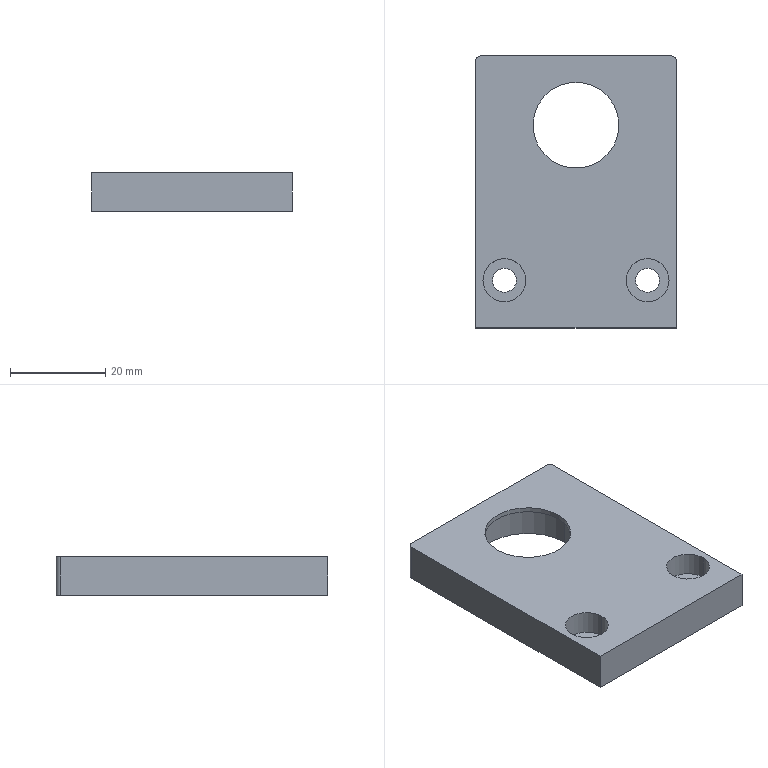Part | SolidWorks | features ICE 2, Extrusion 1 | 1 solid | 23 faces | box 42 x 57 x 8 mm | volume 15479 mm3 | cylinder 14 | plane 9 | commonest cylinder face diameters 5 x4 9 x4 2 x2 18 x2 22 x2
STEP:
#1=CARTESIAN_POINT('',(11.,14.,7.));
#2=VERTEX_POINT('',#1);
#3=CARTESIAN_POINT('',(-11.,14.,7.));
#4=VERTEX_POINT('',#3);
#5=CARTESIAN_POINT('',(0.,14.,7.));
#6=DIRECTION('',(0.,0.,-1.));
#7=DIRECTION('',(-1.,0.,0.));
#8=AXIS2_PLACEMENT_3D('',#5,#6,#7);
#9=CIRCLE('',#8,11.);
#10=EDGE_CURVE('',#2,#4,#9,.T.);
#11=ORIENTED_EDGE('',*,*,#10,.F.);
#12=CARTESIAN_POINT('',(11.,14.,0.));
#13=VERTEX_POINT('',#12);
#14=CARTESIAN_POINT('',(11.,14.,7.));
#15=DIRECTION('',(0.,0.,-1.));
#16=VECTOR('',#15,1000.);
#17=LINE('',#14,#16);
#18=EDGE_CURVE('',#2,#13,#17,.T.);
#19=ORIENTED_EDGE('',*,*,#18,.T.);
#20=CARTESIAN_POINT('',(-11.,14.,0.));
#21=VERTEX_POINT('',#20);
#22=CARTESIAN_POINT('',(0.,14.,0.));
#23=DIRECTION('',(0.,0.,-1.));
#24=DIRECTION('',(-1.,0.,0.));
#25=AXIS2_PLACEMENT_3D('',#22,#23,#24);
#26=CIRCLE('',#25,11.);
#27=EDGE_CURVE('',#13,#21,#26,.T.);
#28=ORIENTED_EDGE('',*,*,#27,.T.);
#29=CARTESIAN_POINT('',(-11.,14.,7.));
#30=DIRECTION('',(0.,0.,-1.));
#31=VECTOR('',#30,1000.);
#32=LINE('',#29,#31);
#33=EDGE_CURVE('',#4,#21,#32,.T.);
#34=ORIENTED_EDGE('',*,*,#33,.F.);
#35=EDGE_LOOP('',(#11,#19,#28,#34));
#36=FACE_OUTER_BOUND('',#35,.T.);
#37=CARTESIAN_POINT('',(0.,14.,7.));
#38=DIRECTION('',(0.,0.,-1.));
#39=DIRECTION('',(-1.,0.,0.));
#40=AXIS2_PLACEMENT_3D('',#37,#38,#39);
#41=CYLINDRICAL_SURFACE('',#40,11.);
#42=ADVANCED_FACE('',(#36),#41,.F.);
#43=CARTESIAN_POINT('',(10.5,-18.5,3.));
#44=VERTEX_POINT('',#43);
#45=CARTESIAN_POINT('',(19.5,-18.5,3.));
#46=VERTEX_POINT('',#45);
#47=CARTESIAN_POINT('',(15.,-18.5,3.));
#48=DIRECTION('',(0.,0.,1.));
#49=DIRECTION('',(1.,0.,0.));
#50=AXIS2_PLACEMENT_3D('',#47,#48,#49);
#51=CIRCLE('',#50,4.5);
#52=EDGE_CURVE('',#44,#46,#51,.T.);
#53=ORIENTED_EDGE('',*,*,#52,.F.);
#54=CARTESIAN_POINT('',(10.5,-18.5,8.));
#55=VERTEX_POINT('',#54);
#56=CARTESIAN_POINT('',(10.5,-18.5,3.));
#57=DIRECTION('',(0.,0.,1.));
#58=VECTOR('',#57,1000.);
#59=LINE('',#56,#58);
#60=EDGE_CURVE('',#44,#55,#59,.T.);
#61=ORIENTED_EDGE('',*,*,#60,.T.);
#62=CARTESIAN_POINT('',(19.5,-18.5,8.));
#63=VERTEX_POINT('',#62);
#64=CARTESIAN_POINT('',(15.,-18.5,8.));
#65=DIRECTION('',(0.,0.,1.));
#66=DIRECTION('',(1.,0.,0.));
#67=AXIS2_PLACEMENT_3D('',#64,#65,#66);
#68=CIRCLE('',#67,4.5);
#69=EDGE_CURVE('',#55,#63,#68,.T.);
#70=ORIENTED_EDGE('',*,*,#69,.T.);
#71=CARTESIAN_POINT('',(19.5,-18.5,3.));
#72=DIRECTION('',(0.,0.,1.));
#73=VECTOR('',#72,1000.);
#74=LINE('',#71,#73);
#75=EDGE_CURVE('',#46,#63,#74,.T.);
#76=ORIENTED_EDGE('',*,*,#75,.F.);
#77=EDGE_LOOP('',(#53,#61,#70,#76));
#78=FACE_OUTER_BOUND('',#77,.T.);
#79=CARTESIAN_POINT('',(15.,-18.5,3.));
#80=DIRECTION('',(0.,0.,1.));
#81=DIRECTION('',(1.,0.,0.));
#82=AXIS2_PLACEMENT_3D('',#79,#80,#81);
#83=CYLINDRICAL_SURFACE('',#82,4.5);
#84=ADVANCED_FACE('',(#78),#83,.F.);
#85=CARTESIAN_POINT('',(-19.5,-18.5,3.));
#86=VERTEX_POINT('',#85);
#87=CARTESIAN_POINT('',(-10.5,-18.5,3.));
#88=VERTEX_POINT('',#87);
#89=CARTESIAN_POINT('',(-15.,-18.5,3.));
#90=DIRECTION('',(0.,0.,1.));
#91=DIRECTION('',(1.,0.,0.));
#92=AXIS2_PLACEMENT_3D('',#89,#90,#91);
#93=CIRCLE('',#92,4.5);
#94=EDGE_CURVE('',#86,#88,#93,.T.);
#95=ORIENTED_EDGE('',*,*,#94,.F.);
#96=CARTESIAN_POINT('',(-19.5,-18.5,8.));
#97=VERTEX_POINT('',#96);
#98=CARTESIAN_POINT('',(-19.5,-18.5,3.));
#99=DIRECTION('',(0.,0.,1.));
#100=VECTOR('',#99,1000.);
#101=LINE('',#98,#100);
#102=EDGE_CURVE('',#86,#97,#101,.T.);
#103=ORIENTED_EDGE('',*,*,#102,.T.);
#104=CARTESIAN_POINT('',(-10.5,-18.5,8.));
#105=VERTEX_POINT('',#104);
#106=CARTESIAN_POINT('',(-15.,-18.5,8.));
#107=DIRECTION('',(0.,0.,1.));
#108=DIRECTION('',(1.,0.,0.));
#109=AXIS2_PLACEMENT_3D('',#106,#107,#108);
#110=CIRCLE('',#109,4.5);
#111=EDGE_CURVE('',#97,#105,#110,.T.);
#112=ORIENTED_EDGE('',*,*,#111,.T.);
#113=CARTESIAN_POINT('',(-10.5,-18.5,3.));
#114=DIRECTION('',(0.,0.,1.));
#115=VECTOR('',#114,1000.);
#116=LINE('',#113,#115);
#117=EDGE_CURVE('',#88,#105,#116,.T.);
#118=ORIENTED_EDGE('',*,*,#117,.F.);
#119=EDGE_LOOP('',(#95,#103,#112,#118));
#120=FACE_OUTER_BOUND('',#119,.T.);
#121=CARTESIAN_POINT('',(-15.,-18.5,3.));
#122=DIRECTION('',(0.,0.,1.));
#123=DIRECTION('',(1.,0.,0.));
#124=AXIS2_PLACEMENT_3D('',#121,#122,#123);
#125=CYLINDRICAL_SURFACE('',#124,4.5);
#126=ADVANCED_FACE('',(#120),#125,.F.);
#127=CARTESIAN_POINT('',(-17.5,-18.5,3.));
#128=VERTEX_POINT('',#127);
#129=CARTESIAN_POINT('',(-12.5,-18.5,3.));
#130=VERTEX_POINT('',#129);
#131=CARTESIAN_POINT('',(-15.,-18.5,3.));
#132=DIRECTION('',(0.,0.,1.));
#133=DIRECTION('',(1.,0.,0.));
#134=AXIS2_PLACEMENT_3D('',#131,#132,#133);
#135=CIRCLE('',#134,2.5);
#136=EDGE_CURVE('',#128,#130,#135,.T.);
#137=ORIENTED_EDGE('',*,*,#136,.T.);
#138=CARTESIAN_POINT('',(-12.5,-18.5,0.));
#139=VERTEX_POINT('',#138);
#140=CARTESIAN_POINT('',(-12.5,-18.5,8.));
#141=DIRECTION('',(0.,0.,-1.));
#142=VECTOR('',#141,1000.);
#143=LINE('',#140,#142);
#144=EDGE_CURVE('',#130,#139,#143,.T.);
#145=ORIENTED_EDGE('',*,*,#144,.T.);
#146=CARTESIAN_POINT('',(-17.5,-18.5,0.));
#147=VERTEX_POINT('',#146);
#148=CARTESIAN_POINT('',(-15.,-18.5,0.));
#149=DIRECTION('',(0.,0.,1.));
#150=DIRECTION('',(1.,0.,0.));
#151=AXIS2_PLACEMENT_3D('',#148,#149,#150);
#152=CIRCLE('',#151,2.5);
#153=EDGE_CURVE('',#147,#139,#152,.T.);
#154=ORIENTED_EDGE('',*,*,#153,.F.);
#155=CARTESIAN_POINT('',(-17.5,-18.5,8.));
#156=DIRECTION('',(0.,0.,-1.));
#157=VECTOR('',#156,1000.);
#158=LINE('',#155,#157);
#159=EDGE_CURVE('',#128,#147,#158,.T.);
#160=ORIENTED_EDGE('',*,*,#159,.F.);
#161=EDGE_LOOP('',(#137,#145,#154,#160));
#162=FACE_OUTER_BOUND('',#161,.T.);
#163=CARTESIAN_POINT('',(-15.,-18.5,8.));
#164=DIRECTION('',(0.,0.,-1.));
#165=DIRECTION('',(-1.,0.,0.));
#166=AXIS2_PLACEMENT_3D('',#163,#164,#165);
#167=CYLINDRICAL_SURFACE('',#166,2.5);
#168=ADVANCED_FACE('',(#162),#167,.F.);
#169=CARTESIAN_POINT('',(12.5,-18.5,3.));
#170=VERTEX_POINT('',#169);
#171=CARTESIAN_POINT('',(17.5,-18.5,3.));
#172=VERTEX_POINT('',#171);
#173=CARTESIAN_POINT('',(15.,-18.5,3.));
#174=DIRECTION('',(0.,0.,1.));
#175=DIRECTION('',(1.,0.,0.));
#176=AXIS2_PLACEMENT_3D('',#173,#174,#175);
#177=CIRCLE('',#176,2.5);
#178=EDGE_CURVE('',#170,#172,#177,.T.);
#179=ORIENTED_EDGE('',*,*,#178,.T.);
#180=CARTESIAN_POINT('',(17.5,-18.5,0.));
#181=VERTEX_POINT('',#180);
#182=CARTESIAN_POINT('',(17.5,-18.5,8.));
#183=DIRECTION('',(0.,0.,-1.));
#184=VECTOR('',#183,1000.);
#185=LINE('',#182,#184);
#186=EDGE_CURVE('',#172,#181,#185,.T.);
#187=ORIENTED_EDGE('',*,*,#186,.T.);
#188=CARTESIAN_POINT('',(12.5,-18.5,0.));
#189=VERTEX_POINT('',#188);
#190=CARTESIAN_POINT('',(15.,-18.5,0.));
#191=DIRECTION('',(0.,0.,1.));
#192=DIRECTION('',(1.,0.,0.));
#193=AXIS2_PLACEMENT_3D('',#190,#191,#192);
#194=CIRCLE('',#193,2.5);
#195=EDGE_CURVE('',#189,#181,#194,.T.);
#196=ORIENTED_EDGE('',*,*,#195,.F.);
#197=CARTESIAN_POINT('',(12.5,-18.5,8.));
#198=DIRECTION('',(0.,0.,-1.));
#199=VECTOR('',#198,1000.);
#200=LINE('',#197,#199);
#201=EDGE_CURVE('',#170,#189,#200,.T.);
#202=ORIENTED_EDGE('',*,*,#201,.F.);
#203=EDGE_LOOP('',(#179,#187,#196,#202));
#204=FACE_OUTER_BOUND('',#203,.T.);
#205=CARTESIAN_POINT('',(15.,-18.5,8.));
#206=DIRECTION('',(0.,0.,-1.));
#207=DIRECTION('',(-1.,0.,0.));
#208=AXIS2_PLACEMENT_3D('',#205,#206,#207);
#209=CYLINDRICAL_SURFACE('',#208,2.5);
#210=ADVANCED_FACE('',(#204),#209,.F.);
#211=CARTESIAN_POINT('',(-9.,14.,8.));
#212=VERTEX_POINT('',#211);
#213=CARTESIAN_POINT('',(9.,14.,8.));
#214=VERTEX_POINT('',#213);
#215=CARTESIAN_POINT('',(0.,14.,8.));
#216=DIRECTION('',(0.,0.,1.));
#217=DIRECTION('',(1.,0.,0.));
#218=AXIS2_PLACEMENT_3D('',#215,#216,#217);
#219=CIRCLE('',#218,9.);
#220=EDGE_CURVE('',#212,#214,#219,.T.);
#221=ORIENTED_EDGE('',*,*,#220,.T.);
#222=CARTESIAN_POINT('',(9.,14.,7.));
#223=VERTEX_POINT('',#222);
#224=CARTESIAN_POINT('',(9.,14.,8.));
#225=DIRECTION('',(0.,0.,-1.));
#226=VECTOR('',#225,1000.);
#227=LINE('',#224,#226);
#228=EDGE_CURVE('',#214,#223,#227,.T.);
#229=ORIENTED_EDGE('',*,*,#228,.T.);
#230=CARTESIAN_POINT('',(-9.,14.,7.));
#231=VERTEX_POINT('',#230);
#232=CARTESIAN_POINT('',(0.,14.,7.));
#233=DIRECTION('',(0.,0.,-1.));
#234=DIRECTION('',(-1.,0.,0.));
#235=AXIS2_PLACEMENT_3D('',#232,#233,#234);
#236=CIRCLE('',#235,9.);
#237=EDGE_CURVE('',#223,#231,#236,.T.);
#238=ORIENTED_EDGE('',*,*,#237,.T.);
#239=CARTESIAN_POINT('',(-9.,14.,8.));
#240=DIRECTION('',(0.,0.,-1.));
#241=VECTOR('',#240,1000.);
#242=LINE('',#239,#241);
#243=EDGE_CURVE('',#212,#231,#242,.T.);
#244=ORIENTED_EDGE('',*,*,#243,.F.);
#245=EDGE_LOOP('',(#221,#229,#238,#244));
#246=FACE_OUTER_BOUND('',#245,.T.);
#247=CARTESIAN_POINT('',(0.,14.,8.));
#248=DIRECTION('',(0.,0.,-1.));
#249=DIRECTION('',(-1.,0.,0.));
#250=AXIS2_PLACEMENT_3D('',#247,#248,#249);
#251=CYLINDRICAL_SURFACE('',#250,9.);
#252=ADVANCED_FACE('',(#246),#251,.F.);
#253=ORIENTED_EDGE('',*,*,#228,.F.);
#254=CARTESIAN_POINT('',(0.,14.,8.));
#255=DIRECTION('',(0.,0.,1.));
#256=DIRECTION('',(1.,0.,0.));
#257=AXIS2_PLACEMENT_3D('',#254,#255,#256);
#258=CIRCLE('',#257,9.);
#259=EDGE_CURVE('',#214,#212,#258,.T.);
#260=ORIENTED_EDGE('',*,*,#259,.T.);
#261=ORIENTED_EDGE('',*,*,#243,.T.);
#262=CARTESIAN_POINT('',(0.,14.,7.));
#263=DIRECTION('',(0.,0.,-1.));
#264=DIRECTION('',(-1.,0.,0.));
#265=AXIS2_PLACEMENT_3D('',#262,#263,#264);
#266=CIRCLE('',#265,9.);
#267=EDGE_CURVE('',#231,#223,#266,.T.);
#268=ORIENTED_EDGE('',*,*,#267,.T.);
#269=EDGE_LOOP('',(#253,#260,#261,#268));
#270=FACE_OUTER_BOUND('',#269,.T.);
#271=CARTESIAN_POINT('',(0.,14.,8.));
#272=DIRECTION('',(0.,0.,-1.));
#273=DIRECTION('',(-1.,0.,0.));
#274=AXIS2_PLACEMENT_3D('',#271,#272,#273);
#275=CYLINDRICAL_SURFACE('',#274,9.);
#276=ADVANCED_FACE('',(#270),#275,.F.);
#277=ORIENTED_EDGE('',*,*,#186,.F.);
#278=CARTESIAN_POINT('',(15.,-18.5,3.));
#279=DIRECTION('',(0.,0.,1.));
#280=DIRECTION('',(1.,0.,0.));
#281=AXIS2_PLACEMENT_3D('',#278,#279,#280);
#282=CIRCLE('',#281,2.5);
#283=EDGE_CURVE('',#172,#170,#282,.T.);
#284=ORIENTED_EDGE('',*,*,#283,.T.);
#285=ORIENTED_EDGE('',*,*,#201,.T.);
#286=CARTESIAN_POINT('',(15.,-18.5,0.));
#287=DIRECTION('',(0.,0.,1.));
#288=DIRECTION('',(1.,0.,0.));
#289=AXIS2_PLACEMENT_3D('',#286,#287,#288);
#290=CIRCLE('',#289,2.5);
#291=EDGE_CURVE('',#181,#189,#290,.T.);
#292=ORIENTED_EDGE('',*,*,#291,.F.);
#293=EDGE_LOOP('',(#277,#284,#285,#292));
#294=FACE_OUTER_BOUND('',#293,.T.);
#295=CARTESIAN_POINT('',(15.,-18.5,8.));
#296=DIRECTION('',(0.,0.,-1.));
#297=DIRECTION('',(-1.,0.,0.));
#298=AXIS2_PLACEMENT_3D('',#295,#296,#297);
#299=CYLINDRICAL_SURFACE('',#298,2.5);
#300=ADVANCED_FACE('',(#294),#299,.F.);
#301=ORIENTED_EDGE('',*,*,#144,.F.);
#302=CARTESIAN_POINT('',(-15.,-18.5,3.));
#303=DIRECTION('',(0.,0.,1.));
#304=DIRECTION('',(1.,0.,0.));
#305=AXIS2_PLACEMENT_3D('',#302,#303,#304);
#306=CIRCLE('',#305,2.5);
#307=EDGE_CURVE('',#130,#128,#306,.T.);
#308=ORIENTED_EDGE('',*,*,#307,.T.);
#309=ORIENTED_EDGE('',*,*,#159,.T.);
#310=CARTESIAN_POINT('',(-15.,-18.5,0.));
#311=DIRECTION('',(0.,0.,1.));
#312=DIRECTION('',(1.,0.,0.));
#313=AXIS2_PLACEMENT_3D('',#310,#311,#312);
#314=CIRCLE('',#313,2.5);
#315=EDGE_CURVE('',#139,#147,#314,.T.);
#316=ORIENTED_EDGE('',*,*,#315,.F.);
#317=EDGE_LOOP('',(#301,#308,#309,#316));
#318=FACE_OUTER_BOUND('',#317,.T.);
#319=CARTESIAN_POINT('',(-15.,-18.5,8.));
#320=DIRECTION('',(0.,0.,-1.));
#321=DIRECTION('',(-1.,0.,0.));
#322=AXIS2_PLACEMENT_3D('',#319,#320,#321);
#323=CYLINDRICAL_SURFACE('',#322,2.5);
#324=ADVANCED_FACE('',(#318),#323,.F.);
#325=CARTESIAN_POINT('',(15.,-18.5,8.));
#326=DIRECTION('',(0.,0.,1.));
#327=DIRECTION('',(1.,0.,0.));
#328=AXIS2_PLACEMENT_3D('',#325,#326,#327);
#329=CIRCLE('',#328,4.5);
#330=EDGE_CURVE('',#63,#55,#329,.T.);
#331=ORIENTED_EDGE('',*,*,#330,.F.);
#332=ORIENTED_EDGE('',*,*,#69,.F.);
#333=EDGE_LOOP('',(#331,#332));
#334=FACE_BOUND('',#333,.T.);
#335=CARTESIAN_POINT('',(-15.,-18.5,8.));
#336=DIRECTION('',(0.,0.,1.));
#337=DIRECTION('',(1.,0.,0.));
#338=AXIS2_PLACEMENT_3D('',#335,#336,#337);
#339=CIRCLE('',#338,4.5);
#340=EDGE_CURVE('',#105,#97,#339,.T.);
#341=ORIENTED_EDGE('',*,*,#340,.F.);
#342=ORIENTED_EDGE('',*,*,#111,.F.);
#343=EDGE_LOOP('',(#341,#342));
#344=FACE_BOUND('',#343,.T.);
#345=CARTESIAN_POINT('',(21.,-28.5,8.));
#346=VERTEX_POINT('',#345);
#347=CARTESIAN_POINT('',(21.,27.5,8.));
#348=VERTEX_POINT('',#347);
#349=CARTESIAN_POINT('',(21.,27.5,8.));
#350=DIRECTION('',(0.,1.,0.));
#351=VECTOR('',#350,1000.);
#352=LINE('',#349,#351);
#353=EDGE_CURVE('',#346,#348,#352,.T.);
#354=ORIENTED_EDGE('',*,*,#353,.T.);
#355=CARTESIAN_POINT('',(20.,28.5,8.));
#356=VERTEX_POINT('',#355);
#357=CARTESIAN_POINT('',(20.,27.5,8.));
#358=DIRECTION('',(0.,0.,1.));
#359=DIRECTION('',(-1.,0.,0.));
#360=AXIS2_PLACEMENT_3D('',#357,#358,#359);
#361=CIRCLE('',#360,1.);
#362=EDGE_CURVE('',#348,#356,#361,.T.);
#363=ORIENTED_EDGE('',*,*,#362,.T.);
#364=CARTESIAN_POINT('',(-20.,28.5,8.));
#365=VERTEX_POINT('',#364);
#366=CARTESIAN_POINT('',(-20.,28.5,8.));
#367=DIRECTION('',(-1.,0.,0.));
#368=VECTOR('',#367,1000.);
#369=LINE('',#366,#368);
#370=EDGE_CURVE('',#356,#365,#369,.T.);
#371=ORIENTED_EDGE('',*,*,#370,.T.);
#372=CARTESIAN_POINT('',(-21.,27.5,8.));
#373=VERTEX_POINT('',#372);
#374=CARTESIAN_POINT('',(-20.,27.5,8.));
#375=DIRECTION('',(0.,0.,1.));
#376=DIRECTION('',(1.,0.,0.));
#377=AXIS2_PLACEMENT_3D('',#374,#375,#376);
#378=CIRCLE('',#377,1.);
#379=EDGE_CURVE('',#365,#373,#378,.T.);
#380=ORIENTED_EDGE('',*,*,#379,.T.);
#381=CARTESIAN_POINT('',(-21.,-28.5,8.));
#382=VERTEX_POINT('',#381);
#383=CARTESIAN_POINT('',(-21.,27.5,8.));
#384=DIRECTION('',(0.,-1.,0.));
#385=VECTOR('',#384,1000.);
#386=LINE('',#383,#385);
#387=EDGE_CURVE('',#373,#382,#386,.T.);
#388=ORIENTED_EDGE('',*,*,#387,.T.);
#389=CARTESIAN_POINT('',(-21.,-28.5,8.));
#390=DIRECTION('',(1.,0.,0.));
#391=VECTOR('',#390,1000.);
#392=LINE('',#389,#391);
#393=EDGE_CURVE('',#382,#346,#392,.T.);
#394=ORIENTED_EDGE('',*,*,#393,.T.);
#395=EDGE_LOOP('',(#354,#363,#371,#380,#388,#394));
#396=FACE_OUTER_BOUND('',#395,.T.);
#397=ORIENTED_EDGE('',*,*,#220,.F.);
#398=ORIENTED_EDGE('',*,*,#259,.F.);
#399=EDGE_LOOP('',(#397,#398));
#400=FACE_BOUND('',#399,.T.);
#401=CARTESIAN_POINT('',(-20.,27.5,8.));
#402=DIRECTION('',(0.,0.,1.));
#403=DIRECTION('',(1.,0.,0.));
#404=AXIS2_PLACEMENT_3D('',#401,#402,#403);
#405=PLANE('',#404);
#406=ADVANCED_FACE('',(#334,#344,#396,#400),#405,.T.);
#407=CARTESIAN_POINT('',(0.,14.,0.));
#408=DIRECTION('',(0.,0.,-1.));
#409=DIRECTION('',(-1.,0.,0.));
#410=AXIS2_PLACEMENT_3D('',#407,#408,#409);
#411=CIRCLE('',#410,11.);
#412=EDGE_CURVE('',#21,#13,#411,.T.);
#413=ORIENTED_EDGE('',*,*,#412,.F.);
#414=ORIENTED_EDGE('',*,*,#27,.F.);
#415=EDGE_LOOP('',(#413,#414));
#416=FACE_BOUND('',#415,.T.);
#417=ORIENTED_EDGE('',*,*,#153,.T.);
#418=ORIENTED_EDGE('',*,*,#315,.T.);
#419=EDGE_LOOP('',(#417,#418));
#420=FACE_BOUND('',#419,.T.);
#421=CARTESIAN_POINT('',(21.,-28.5,0.));
#422=VERTEX_POINT('',#421);
#423=CARTESIAN_POINT('',(21.,27.5,0.));
#424=VERTEX_POINT('',#423);
#425=CARTESIAN_POINT('',(21.,27.5,0.));
#426=DIRECTION('',(0.,1.,0.));
#427=VECTOR('',#426,1000.);
#428=LINE('',#425,#427);
#429=EDGE_CURVE('',#422,#424,#428,.T.);
#430=ORIENTED_EDGE('',*,*,#429,.F.);
#431=CARTESIAN_POINT('',(-21.,-28.5,0.));
#432=VERTEX_POINT('',#431);
#433=CARTESIAN_POINT('',(-21.,-28.5,0.));
#434=DIRECTION('',(1.,0.,0.));
#435=VECTOR('',#434,1000.);
#436=LINE('',#433,#435);
#437=EDGE_CURVE('',#432,#422,#436,.T.);
#438=ORIENTED_EDGE('',*,*,#437,.F.);
#439=CARTESIAN_POINT('',(-21.,27.5,0.));
#440=VERTEX_POINT('',#439);
#441=CARTESIAN_POINT('',(-21.,27.5,0.));
#442=DIRECTION('',(0.,-1.,0.));
#443=VECTOR('',#442,1000.);
#444=LINE('',#441,#443);
#445=EDGE_CURVE('',#440,#432,#444,.T.);
#446=ORIENTED_EDGE('',*,*,#445,.F.);
#447=CARTESIAN_POINT('',(-20.,28.5,0.));
#448=VERTEX_POINT('',#447);
#449=CARTESIAN_POINT('',(-20.,27.5,0.));
#450=DIRECTION('',(0.,0.,1.));
#451=DIRECTION('',(1.,0.,0.));
#452=AXIS2_PLACEMENT_3D('',#449,#450,#451);
#453=CIRCLE('',#452,1.);
#454=EDGE_CURVE('',#448,#440,#453,.T.);
#455=ORIENTED_EDGE('',*,*,#454,.F.);
#456=CARTESIAN_POINT('',(20.,28.5,0.));
#457=VERTEX_POINT('',#456);
#458=CARTESIAN_POINT('',(-20.,28.5,0.));
#459=DIRECTION('',(-1.,0.,0.));
#460=VECTOR('',#459,1000.);
#461=LINE('',#458,#460);
#462=EDGE_CURVE('',#457,#448,#461,.T.);
#463=ORIENTED_EDGE('',*,*,#462,.F.);
#464=CARTESIAN_POINT('',(20.,27.5,0.));
#465=DIRECTION('',(0.,0.,1.));
#466=DIRECTION('',(-1.,0.,0.));
#467=AXIS2_PLACEMENT_3D('',#464,#465,#466);
#468=CIRCLE('',#467,1.);
#469=EDGE_CURVE('',#424,#457,#468,.T.);
#470=ORIENTED_EDGE('',*,*,#469,.F.);
#471=EDGE_LOOP('',(#430,#438,#446,#455,#463,#470));
#472=FACE_OUTER_BOUND('',#471,.T.);
#473=ORIENTED_EDGE('',*,*,#195,.T.);
#474=ORIENTED_EDGE('',*,*,#291,.T.);
#475=EDGE_LOOP('',(#473,#474));
#476=FACE_BOUND('',#475,.T.);
#477=CARTESIAN_POINT('',(-20.,27.5,0.));
#478=DIRECTION('',(0.,0.,1.));
#479=DIRECTION('',(1.,0.,0.));
#480=AXIS2_PLACEMENT_3D('',#477,#478,#479);
#481=PLANE('',#480);
#482=ADVANCED_FACE('',(#416,#420,#472,#476),#481,.F.);
#483=ORIENTED_EDGE('',*,*,#429,.T.);
#484=CARTESIAN_POINT('',(21.,27.5,8.));
#485=DIRECTION('',(0.,0.,-1.));
#486=VECTOR('',#485,1000.);
#487=LINE('',#484,#486);
#488=EDGE_CURVE('',#348,#424,#487,.T.);
#489=ORIENTED_EDGE('',*,*,#488,.F.);
#490=ORIENTED_EDGE('',*,*,#353,.F.);
#491=CARTESIAN_POINT('',(21.,-28.5,8.));
#492=DIRECTION('',(0.,0.,-1.));
#493=VECTOR('',#492,1000.);
#494=LINE('',#491,#493);
#495=EDGE_CURVE('',#346,#422,#494,.T.);
#496=ORIENTED_EDGE('',*,*,#495,.T.);
#497=EDGE_LOOP('',(#483,#489,#490,#496));
#498=FACE_OUTER_BOUND('',#497,.T.);
#499=CARTESIAN_POINT('',(21.,27.5,8.));
#500=DIRECTION('',(-1.,0.,0.));
#501=DIRECTION('',(0.,-1.,0.));
#502=AXIS2_PLACEMENT_3D('',#499,#500,#501);
#503=PLANE('',#502);
#504=ADVANCED_FACE('',(#498),#503,.F.);
#505=ORIENTED_EDGE('',*,*,#469,.T.);
#506=CARTESIAN_POINT('',(20.,28.5,8.));
#507=DIRECTION('',(0.,0.,-1.));
#508=VECTOR('',#507,1000.);
#509=LINE('',#506,#508);
#510=EDGE_CURVE('',#356,#457,#509,.T.);
#511=ORIENTED_EDGE('',*,*,#510,.F.);
#512=ORIENTED_EDGE('',*,*,#362,.F.);
#513=ORIENTED_EDGE('',*,*,#488,.T.);
#514=EDGE_LOOP('',(#505,#511,#512,#513));
#515=FACE_OUTER_BOUND('',#514,.T.);
#516=CARTESIAN_POINT('',(20.,27.5,8.));
#517=DIRECTION('',(0.,0.,-1.));
#518=DIRECTION('',(-1.,0.,0.));
#519=AXIS2_PLACEMENT_3D('',#516,#517,#518);
#520=CYLINDRICAL_SURFACE('',#519,1.);
#521=ADVANCED_FACE('',(#515),#520,.T.);
#522=ORIENTED_EDGE('',*,*,#462,.T.);
#523=CARTESIAN_POINT('',(-20.,28.5,8.));
#524=DIRECTION('',(0.,0.,-1.));
#525=VECTOR('',#524,1000.);
#526=LINE('',#523,#525);
#527=EDGE_CURVE('',#365,#448,#526,.T.);
#528=ORIENTED_EDGE('',*,*,#527,.F.);
#529=ORIENTED_EDGE('',*,*,#370,.F.);
#530=ORIENTED_EDGE('',*,*,#510,.T.);
#531=EDGE_LOOP('',(#522,#528,#529,#530));
#532=FACE_OUTER_BOUND('',#531,.T.);
#533=CARTESIAN_POINT('',(-20.,28.5,8.));
#534=DIRECTION('',(0.,-1.,0.));
#535=DIRECTION('',(0.,0.,-1.));
#536=AXIS2_PLACEMENT_3D('',#533,#534,#535);
#537=PLANE('',#536);
#538=ADVANCED_FACE('',(#532),#537,.F.);
#539=ORIENTED_EDGE('',*,*,#454,.T.);
#540=CARTESIAN_POINT('',(-21.,27.5,8.));
#541=DIRECTION('',(0.,0.,-1.));
#542=VECTOR('',#541,1000.);
#543=LINE('',#540,#542);
#544=EDGE_CURVE('',#373,#440,#543,.T.);
#545=ORIENTED_EDGE('',*,*,#544,.F.);
#546=ORIENTED_EDGE('',*,*,#379,.F.);
#547=ORIENTED_EDGE('',*,*,#527,.T.);
#548=EDGE_LOOP('',(#539,#545,#546,#547));
#549=FACE_OUTER_BOUND('',#548,.T.);
#550=CARTESIAN_POINT('',(-20.,27.5,8.));
#551=DIRECTION('',(0.,0.,-1.));
#552=DIRECTION('',(-1.,0.,0.));
#553=AXIS2_PLACEMENT_3D('',#550,#551,#552);
#554=CYLINDRICAL_SURFACE('',#553,1.);
#555=ADVANCED_FACE('',(#549),#554,.T.);
#556=ORIENTED_EDGE('',*,*,#445,.T.);
#557=CARTESIAN_POINT('',(-21.,-28.5,8.));
#558=DIRECTION('',(0.,0.,-1.));
#559=VECTOR('',#558,1000.);
#560=LINE('',#557,#559);
#561=EDGE_CURVE('',#382,#432,#560,.T.);
#562=ORIENTED_EDGE('',*,*,#561,.F.);
#563=ORIENTED_EDGE('',*,*,#387,.F.);
#564=ORIENTED_EDGE('',*,*,#544,.T.);
#565=EDGE_LOOP('',(#556,#562,#563,#564));
#566=FACE_OUTER_BOUND('',#565,.T.);
#567=CARTESIAN_POINT('',(-21.,27.5,8.));
#568=DIRECTION('',(1.,0.,0.));
#569=DIRECTION('',(0.,1.,0.));
#570=AXIS2_PLACEMENT_3D('',#567,#568,#569);
#571=PLANE('',#570);
#572=ADVANCED_FACE('',(#566),#571,.F.);
#573=ORIENTED_EDGE('',*,*,#437,.T.);
#574=ORIENTED_EDGE('',*,*,#495,.F.);
#575=ORIENTED_EDGE('',*,*,#393,.F.);
#576=ORIENTED_EDGE('',*,*,#561,.T.);
#577=EDGE_LOOP('',(#573,#574,#575,#576));
#578=FACE_OUTER_BOUND('',#577,.T.);
#579=CARTESIAN_POINT('',(-21.,-28.5,8.));
#580=DIRECTION('',(0.,1.,0.));
#581=DIRECTION('',(0.,0.,1.));
#582=AXIS2_PLACEMENT_3D('',#579,#580,#581);
#583=PLANE('',#582);
#584=ADVANCED_FACE('',(#578),#583,.F.);
#585=ORIENTED_EDGE('',*,*,#102,.F.);
#586=CARTESIAN_POINT('',(-15.,-18.5,3.));
#587=DIRECTION('',(0.,0.,1.));
#588=DIRECTION('',(1.,0.,0.));
#589=AXIS2_PLACEMENT_3D('',#586,#587,#588);
#590=CIRCLE('',#589,4.5);
#591=EDGE_CURVE('',#88,#86,#590,.T.);
#592=ORIENTED_EDGE('',*,*,#591,.F.);
#593=ORIENTED_EDGE('',*,*,#117,.T.);
#594=ORIENTED_EDGE('',*,*,#340,.T.);
#595=EDGE_LOOP('',(#585,#592,#593,#594));
#596=FACE_OUTER_BOUND('',#595,.T.);
#597=CARTESIAN_POINT('',(-15.,-18.5,3.));
#598=DIRECTION('',(0.,0.,1.));
#599=DIRECTION('',(1.,0.,0.));
#600=AXIS2_PLACEMENT_3D('',#597,#598,#599);
#601=CYLINDRICAL_SURFACE('',#600,4.5);
#602=ADVANCED_FACE('',(#596),#601,.F.);
#603=ORIENTED_EDGE('',*,*,#136,.F.);
#604=ORIENTED_EDGE('',*,*,#307,.F.);
#605=EDGE_LOOP('',(#603,#604));
#606=FACE_BOUND('',#605,.T.);
#607=ORIENTED_EDGE('',*,*,#591,.T.);
#608=ORIENTED_EDGE('',*,*,#94,.T.);
#609=EDGE_LOOP('',(#607,#608));
#610=FACE_OUTER_BOUND('',#609,.T.);
#611=CARTESIAN_POINT('',(-15.,-18.5,3.));
#612=DIRECTION('',(0.,0.,1.));
#613=DIRECTION('',(1.,0.,0.));
#614=AXIS2_PLACEMENT_3D('',#611,#612,#613);
#615=PLANE('',#614);
#616=ADVANCED_FACE('',(#606,#610),#615,.T.);
#617=ORIENTED_EDGE('',*,*,#60,.F.);
#618=CARTESIAN_POINT('',(15.,-18.5,3.));
#619=DIRECTION('',(0.,0.,1.));
#620=DIRECTION('',(1.,0.,0.));
#621=AXIS2_PLACEMENT_3D('',#618,#619,#620);
#622=CIRCLE('',#621,4.5);
#623=EDGE_CURVE('',#46,#44,#622,.T.);
#624=ORIENTED_EDGE('',*,*,#623,.F.);
#625=ORIENTED_EDGE('',*,*,#75,.T.);
#626=ORIENTED_EDGE('',*,*,#330,.T.);
#627=EDGE_LOOP('',(#617,#624,#625,#626));
#628=FACE_OUTER_BOUND('',#627,.T.);
#629=CARTESIAN_POINT('',(15.,-18.5,3.));
#630=DIRECTION('',(0.,0.,1.));
#631=DIRECTION('',(1.,0.,0.));
#632=AXIS2_PLACEMENT_3D('',#629,#630,#631);
#633=CYLINDRICAL_SURFACE('',#632,4.5);
#634=ADVANCED_FACE('',(#628),#633,.F.);
#635=ORIENTED_EDGE('',*,*,#178,.F.);
#636=ORIENTED_EDGE('',*,*,#283,.F.);
#637=EDGE_LOOP('',(#635,#636));
#638=FACE_BOUND('',#637,.T.);
#639=ORIENTED_EDGE('',*,*,#623,.T.);
#640=ORIENTED_EDGE('',*,*,#52,.T.);
#641=EDGE_LOOP('',(#639,#640));
#642=FACE_OUTER_BOUND('',#641,.T.);
#643=CARTESIAN_POINT('',(15.,-18.5,3.));
#644=DIRECTION('',(0.,0.,1.));
#645=DIRECTION('',(1.,0.,0.));
#646=AXIS2_PLACEMENT_3D('',#643,#644,#645);
#647=PLANE('',#646);
#648=ADVANCED_FACE('',(#638,#642),#647,.T.);
#649=ORIENTED_EDGE('',*,*,#18,.F.);
#650=CARTESIAN_POINT('',(0.,14.,7.));
#651=DIRECTION('',(0.,0.,-1.));
#652=DIRECTION('',(-1.,0.,0.));
#653=AXIS2_PLACEMENT_3D('',#650,#651,#652);
#654=CIRCLE('',#653,11.);
#655=EDGE_CURVE('',#4,#2,#654,.T.);
#656=ORIENTED_EDGE('',*,*,#655,.F.);
#657=ORIENTED_EDGE('',*,*,#33,.T.);
#658=ORIENTED_EDGE('',*,*,#412,.T.);
#659=EDGE_LOOP('',(#649,#656,#657,#658));
#660=FACE_OUTER_BOUND('',#659,.T.);
#661=CARTESIAN_POINT('',(0.,14.,7.));
#662=DIRECTION('',(0.,0.,-1.));
#663=DIRECTION('',(-1.,0.,0.));
#664=AXIS2_PLACEMENT_3D('',#661,#662,#663);
#665=CYLINDRICAL_SURFACE('',#664,11.);
#666=ADVANCED_FACE('',(#660),#665,.F.);
#667=ORIENTED_EDGE('',*,*,#267,.F.);
#668=ORIENTED_EDGE('',*,*,#237,.F.);
#669=EDGE_LOOP('',(#667,#668));
#670=FACE_BOUND('',#669,.T.);
#671=ORIENTED_EDGE('',*,*,#655,.T.);
#672=ORIENTED_EDGE('',*,*,#10,.T.);
#673=EDGE_LOOP('',(#671,#672));
#674=FACE_OUTER_BOUND('',#673,.T.);
#675=CARTESIAN_POINT('',(0.,14.,7.));
#676=DIRECTION('',(0.,0.,-1.));
#677=DIRECTION('',(-1.,0.,0.));
#678=AXIS2_PLACEMENT_3D('',#675,#676,#677);
#679=PLANE('',#678);
#680=ADVANCED_FACE('',(#670,#674),#679,.T.);
#681=CLOSED_SHELL('',(#42,#84,#126,#168,#210,#252,#276,#300,#324,#406,#482,#504,#521,#538,#555,#572,#584,#602,#616,#634,#648,#666,#680));
#682=MANIFOLD_SOLID_BREP('',#681);
#683=CARTESIAN_POINT('',(0.,0.,0.));
#684=DIRECTION('',(0.,0.,1.));
#685=DIRECTION('',(1.,0.,0.));
#686=AXIS2_PLACEMENT_3D('',#683,#684,#685);
#687=(LENGTH_UNIT()NAMED_UNIT(*)SI_UNIT(.MILLI.,.METRE.));
#688=UNCERTAINTY_MEASURE_WITH_UNIT(LENGTH_MEASURE(0.00001),#687,'','');
#689=(NAMED_UNIT(*)PLANE_ANGLE_UNIT()SI_UNIT($,.RADIAN.));
#690=(NAMED_UNIT(*)SI_UNIT($,.STERADIAN.)SOLID_ANGLE_UNIT());
#691=(GEOMETRIC_REPRESENTATION_CONTEXT(3)GLOBAL_UNCERTAINTY_ASSIGNED_CONTEXT((#688))GLOBAL_UNIT_ASSIGNED_CONTEXT((#687,#689,#690))REPRESENTATION_CONTEXT('',''));
#692=ADVANCED_BREP_SHAPE_REPRESENTATION('',(#682,#686),#691);